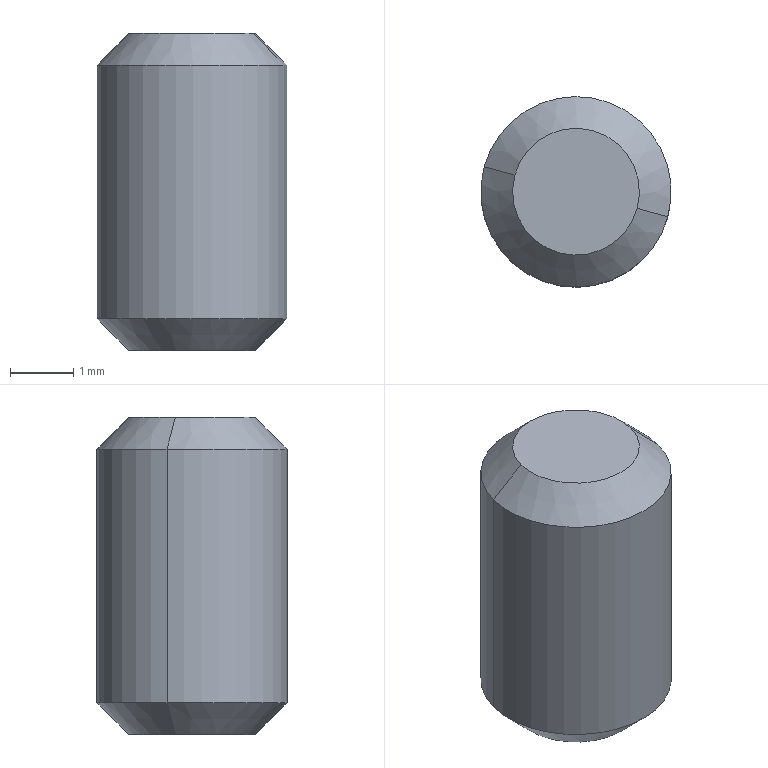Part | SolidWorks | features BaseBody 1 | 1 solid | 8 faces | box 3 x 3 x 5 mm | volume 33.249 mm3 | cone 4 | cylinder 2 | plane 2 | commonest cylinder face diameters 3 x2
STEP:
#1=CARTESIAN_POINT('',(329.335,162.263,-39.));
#2=VERTEX_POINT('',#1);
#3=CARTESIAN_POINT('',(331.265,161.737,-39.));
#4=VERTEX_POINT('',#3);
#5=CARTESIAN_POINT('',(330.3,162.,-39.));
#6=DIRECTION('',(0.,0.,-1.));
#7=DIRECTION('',(-0.9649,0.2627,0.));
#8=AXIS2_PLACEMENT_3D('',#5,#6,#7);
#9=CIRCLE('',#8,1.);
#10=EDGE_CURVE('',#2,#4,#9,.T.);
#11=ORIENTED_EDGE('',*,*,#10,.F.);
#12=CARTESIAN_POINT('',(328.853,162.394,-38.5));
#13=VERTEX_POINT('',#12);
#14=CARTESIAN_POINT('',(329.335,162.263,-39.));
#15=DIRECTION('',(-0.6823,0.1858,0.7071));
#16=VECTOR('',#15,1000.);
#17=LINE('',#14,#16);
#18=EDGE_CURVE('',#2,#13,#17,.T.);
#19=ORIENTED_EDGE('',*,*,#18,.T.);
#20=CARTESIAN_POINT('',(331.747,161.606,-38.5));
#21=VERTEX_POINT('',#20);
#22=CARTESIAN_POINT('',(330.3,162.,-38.5));
#23=DIRECTION('',(0.,0.,1.));
#24=DIRECTION('',(-0.9649,0.2627,0.));
#25=AXIS2_PLACEMENT_3D('',#22,#23,#24);
#26=CIRCLE('',#25,1.5);
#27=EDGE_CURVE('',#21,#13,#26,.T.);
#28=ORIENTED_EDGE('',*,*,#27,.F.);
#29=CARTESIAN_POINT('',(331.265,161.737,-39.));
#30=DIRECTION('',(0.6823,-0.1858,0.7071));
#31=VECTOR('',#30,1000.);
#32=LINE('',#29,#31);
#33=EDGE_CURVE('',#4,#21,#32,.T.);
#34=ORIENTED_EDGE('',*,*,#33,.F.);
#35=EDGE_LOOP('',(#11,#19,#28,#34));
#36=FACE_OUTER_BOUND('',#35,.T.);
#37=CARTESIAN_POINT('',(330.3,162.,-39.));
#38=DIRECTION('',(0.,0.,1.));
#39=DIRECTION('',(0.9649,-0.2627,0.));
#40=AXIS2_PLACEMENT_3D('',#37,#38,#39);
#41=CONICAL_SURFACE('',#40,1.,0.7854);
#42=ADVANCED_FACE('',(#36),#41,.T.);
#43=CARTESIAN_POINT('',(331.265,161.737,-34.));
#44=VERTEX_POINT('',#43);
#45=CARTESIAN_POINT('',(329.335,162.263,-34.));
#46=VERTEX_POINT('',#45);
#47=CARTESIAN_POINT('',(330.3,162.,-34.));
#48=DIRECTION('',(0.,0.,1.));
#49=DIRECTION('',(-0.9649,0.2627,0.));
#50=AXIS2_PLACEMENT_3D('',#47,#48,#49);
#51=CIRCLE('',#50,1.);
#52=EDGE_CURVE('',#44,#46,#51,.T.);
#53=ORIENTED_EDGE('',*,*,#52,.F.);
#54=CARTESIAN_POINT('',(331.747,161.606,-34.5));
#55=VERTEX_POINT('',#54);
#56=CARTESIAN_POINT('',(331.747,161.606,-34.5));
#57=DIRECTION('',(0.6823,-0.1858,-0.7071));
#58=VECTOR('',#57,1000.);
#59=LINE('',#56,#58);
#60=EDGE_CURVE('',#44,#55,#59,.T.);
#61=ORIENTED_EDGE('',*,*,#60,.T.);
#62=CARTESIAN_POINT('',(328.853,162.394,-34.5));
#63=VERTEX_POINT('',#62);
#64=CARTESIAN_POINT('',(330.3,162.,-34.5));
#65=DIRECTION('',(0.,0.,-1.));
#66=DIRECTION('',(-0.9649,0.2627,0.));
#67=AXIS2_PLACEMENT_3D('',#64,#65,#66);
#68=CIRCLE('',#67,1.5);
#69=EDGE_CURVE('',#63,#55,#68,.T.);
#70=ORIENTED_EDGE('',*,*,#69,.F.);
#71=CARTESIAN_POINT('',(328.853,162.394,-34.5));
#72=DIRECTION('',(-0.6823,0.1858,-0.7071));
#73=VECTOR('',#72,1000.);
#74=LINE('',#71,#73);
#75=EDGE_CURVE('',#46,#63,#74,.T.);
#76=ORIENTED_EDGE('',*,*,#75,.F.);
#77=EDGE_LOOP('',(#53,#61,#70,#76));
#78=FACE_OUTER_BOUND('',#77,.T.);
#79=CARTESIAN_POINT('',(330.3,162.,-34.5));
#80=DIRECTION('',(0.,0.,-1.));
#81=DIRECTION('',(-0.9649,0.2627,0.));
#82=AXIS2_PLACEMENT_3D('',#79,#80,#81);
#83=CONICAL_SURFACE('',#82,1.5,0.7854);
#84=ADVANCED_FACE('',(#78),#83,.T.);
#85=ORIENTED_EDGE('',*,*,#27,.T.);
#86=CARTESIAN_POINT('',(328.853,162.394,-39.));
#87=DIRECTION('',(0.,0.,1.));
#88=VECTOR('',#87,1000.);
#89=LINE('',#86,#88);
#90=EDGE_CURVE('',#13,#63,#89,.T.);
#91=ORIENTED_EDGE('',*,*,#90,.T.);
#92=ORIENTED_EDGE('',*,*,#69,.T.);
#93=CARTESIAN_POINT('',(331.747,161.606,-39.));
#94=DIRECTION('',(0.,0.,1.));
#95=VECTOR('',#94,1000.);
#96=LINE('',#93,#95);
#97=EDGE_CURVE('',#21,#55,#96,.T.);
#98=ORIENTED_EDGE('',*,*,#97,.F.);
#99=EDGE_LOOP('',(#85,#91,#92,#98));
#100=FACE_OUTER_BOUND('',#99,.T.);
#101=CARTESIAN_POINT('',(330.3,162.,-39.));
#102=DIRECTION('',(0.,0.,1.));
#103=DIRECTION('',(0.9649,-0.2627,0.));
#104=AXIS2_PLACEMENT_3D('',#101,#102,#103);
#105=CYLINDRICAL_SURFACE('',#104,1.5);
#106=ADVANCED_FACE('',(#100),#105,.T.);
#107=ORIENTED_EDGE('',*,*,#90,.F.);
#108=CARTESIAN_POINT('',(330.3,162.,-38.5));
#109=DIRECTION('',(0.,0.,1.));
#110=DIRECTION('',(-0.9649,0.2627,0.));
#111=AXIS2_PLACEMENT_3D('',#108,#109,#110);
#112=CIRCLE('',#111,1.5);
#113=EDGE_CURVE('',#13,#21,#112,.T.);
#114=ORIENTED_EDGE('',*,*,#113,.T.);
#115=ORIENTED_EDGE('',*,*,#97,.T.);
#116=CARTESIAN_POINT('',(330.3,162.,-34.5));
#117=DIRECTION('',(0.,0.,-1.));
#118=DIRECTION('',(-0.9649,0.2627,0.));
#119=AXIS2_PLACEMENT_3D('',#116,#117,#118);
#120=CIRCLE('',#119,1.5);
#121=EDGE_CURVE('',#55,#63,#120,.T.);
#122=ORIENTED_EDGE('',*,*,#121,.T.);
#123=EDGE_LOOP('',(#107,#114,#115,#122));
#124=FACE_OUTER_BOUND('',#123,.T.);
#125=CARTESIAN_POINT('',(330.3,162.,-39.));
#126=DIRECTION('',(0.,0.,1.));
#127=DIRECTION('',(0.9649,-0.2627,0.));
#128=AXIS2_PLACEMENT_3D('',#125,#126,#127);
#129=CYLINDRICAL_SURFACE('',#128,1.5);
#130=ADVANCED_FACE('',(#124),#129,.T.);
#131=CARTESIAN_POINT('',(330.3,162.,-39.));
#132=DIRECTION('',(0.,0.,-1.));
#133=DIRECTION('',(-0.9649,0.2627,0.));
#134=AXIS2_PLACEMENT_3D('',#131,#132,#133);
#135=CIRCLE('',#134,1.);
#136=EDGE_CURVE('',#4,#2,#135,.T.);
#137=ORIENTED_EDGE('',*,*,#136,.T.);
#138=ORIENTED_EDGE('',*,*,#10,.T.);
#139=EDGE_LOOP('',(#137,#138));
#140=FACE_OUTER_BOUND('',#139,.T.);
#141=CARTESIAN_POINT('',(330.3,162.,-39.));
#142=DIRECTION('',(0.,0.,-1.));
#143=DIRECTION('',(-0.9649,0.2627,0.));
#144=AXIS2_PLACEMENT_3D('',#141,#142,#143);
#145=PLANE('',#144);
#146=ADVANCED_FACE('',(#140),#145,.T.);
#147=CARTESIAN_POINT('',(330.3,162.,-34.));
#148=DIRECTION('',(0.,0.,1.));
#149=DIRECTION('',(-0.9649,0.2627,0.));
#150=AXIS2_PLACEMENT_3D('',#147,#148,#149);
#151=CIRCLE('',#150,1.);
#152=EDGE_CURVE('',#46,#44,#151,.T.);
#153=ORIENTED_EDGE('',*,*,#152,.T.);
#154=ORIENTED_EDGE('',*,*,#52,.T.);
#155=EDGE_LOOP('',(#153,#154));
#156=FACE_OUTER_BOUND('',#155,.T.);
#157=CARTESIAN_POINT('',(330.3,162.,-34.));
#158=DIRECTION('',(0.,0.,-1.));
#159=DIRECTION('',(-0.9649,0.2627,0.));
#160=AXIS2_PLACEMENT_3D('',#157,#158,#159);
#161=PLANE('',#160);
#162=ADVANCED_FACE('',(#156),#161,.F.);
#163=ORIENTED_EDGE('',*,*,#60,.F.);
#164=ORIENTED_EDGE('',*,*,#152,.F.);
#165=ORIENTED_EDGE('',*,*,#75,.T.);
#166=ORIENTED_EDGE('',*,*,#121,.F.);
#167=EDGE_LOOP('',(#163,#164,#165,#166));
#168=FACE_OUTER_BOUND('',#167,.T.);
#169=CARTESIAN_POINT('',(330.3,162.,-34.5));
#170=DIRECTION('',(0.,0.,-1.));
#171=DIRECTION('',(-0.9649,0.2627,0.));
#172=AXIS2_PLACEMENT_3D('',#169,#170,#171);
#173=CONICAL_SURFACE('',#172,1.5,0.7854);
#174=ADVANCED_FACE('',(#168),#173,.T.);
#175=ORIENTED_EDGE('',*,*,#18,.F.);
#176=ORIENTED_EDGE('',*,*,#136,.F.);
#177=ORIENTED_EDGE('',*,*,#33,.T.);
#178=ORIENTED_EDGE('',*,*,#113,.F.);
#179=EDGE_LOOP('',(#175,#176,#177,#178));
#180=FACE_OUTER_BOUND('',#179,.T.);
#181=CARTESIAN_POINT('',(330.3,162.,-39.));
#182=DIRECTION('',(0.,0.,1.));
#183=DIRECTION('',(0.9649,-0.2627,0.));
#184=AXIS2_PLACEMENT_3D('',#181,#182,#183);
#185=CONICAL_SURFACE('',#184,1.,0.7854);
#186=ADVANCED_FACE('',(#180),#185,.T.);
#187=CLOSED_SHELL('',(#42,#84,#106,#130,#146,#162,#174,#186));
#188=MANIFOLD_SOLID_BREP('',#187);
#189=CARTESIAN_POINT('',(0.,0.,0.));
#190=DIRECTION('',(0.,0.,1.));
#191=DIRECTION('',(1.,0.,0.));
#192=AXIS2_PLACEMENT_3D('',#189,#190,#191);
#193=(LENGTH_UNIT()NAMED_UNIT(*)SI_UNIT(.MILLI.,.METRE.));
#194=UNCERTAINTY_MEASURE_WITH_UNIT(LENGTH_MEASURE(0.00001),#193,'','');
#195=(NAMED_UNIT(*)PLANE_ANGLE_UNIT()SI_UNIT($,.RADIAN.));
#196=(NAMED_UNIT(*)SI_UNIT($,.STERADIAN.)SOLID_ANGLE_UNIT());
#197=(GEOMETRIC_REPRESENTATION_CONTEXT(3)GLOBAL_UNCERTAINTY_ASSIGNED_CONTEXT((#194))GLOBAL_UNIT_ASSIGNED_CONTEXT((#193,#195,#196))REPRESENTATION_CONTEXT('',''));
#198=ADVANCED_BREP_SHAPE_REPRESENTATION('',(#188,#192),#197);